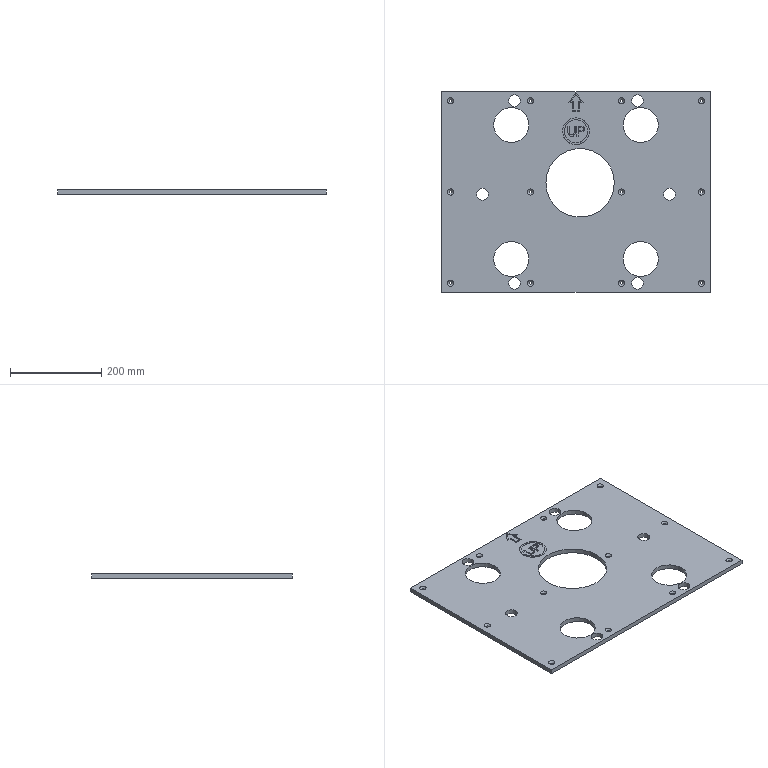Part | STEP file | solid 79 | 1 solid | 114 faces | box 590 x 440 x 10 mm | volume 2194749 mm3 | spline 42 | plane 37 | cylinder 23 | cone 12 | commonest cylinder face diameters 6 x12 26 x6 77 x4 150 x1